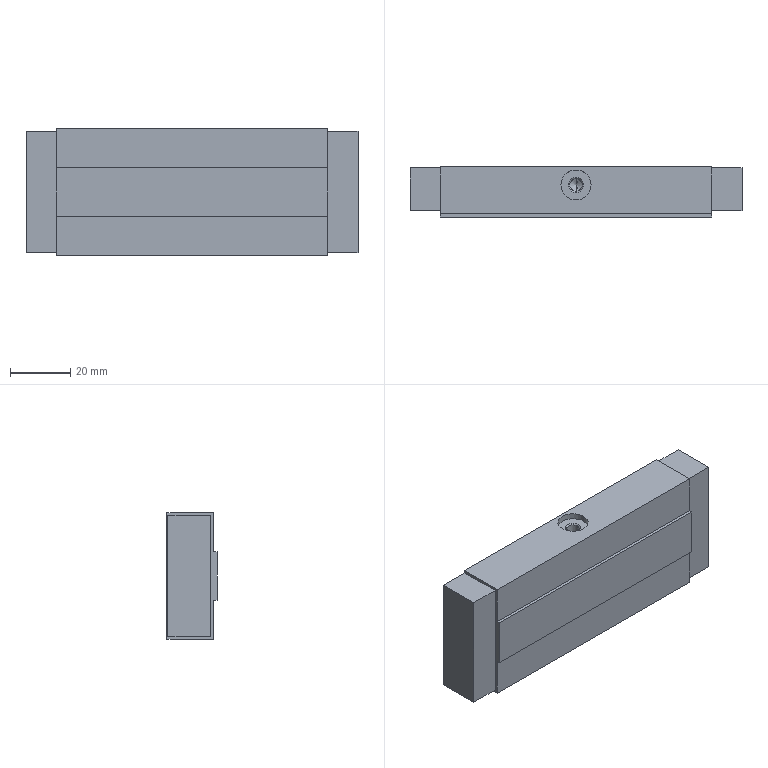Part | SolidWorks | features BaseBody 1 | 1 solid | 62 faces | box 110 x 16.6 x 42 mm | volume 70637 mm3 | cone 24 | plane 22 | cylinder 16 | commonest cylinder face diameters 4.134 x12 10 x4